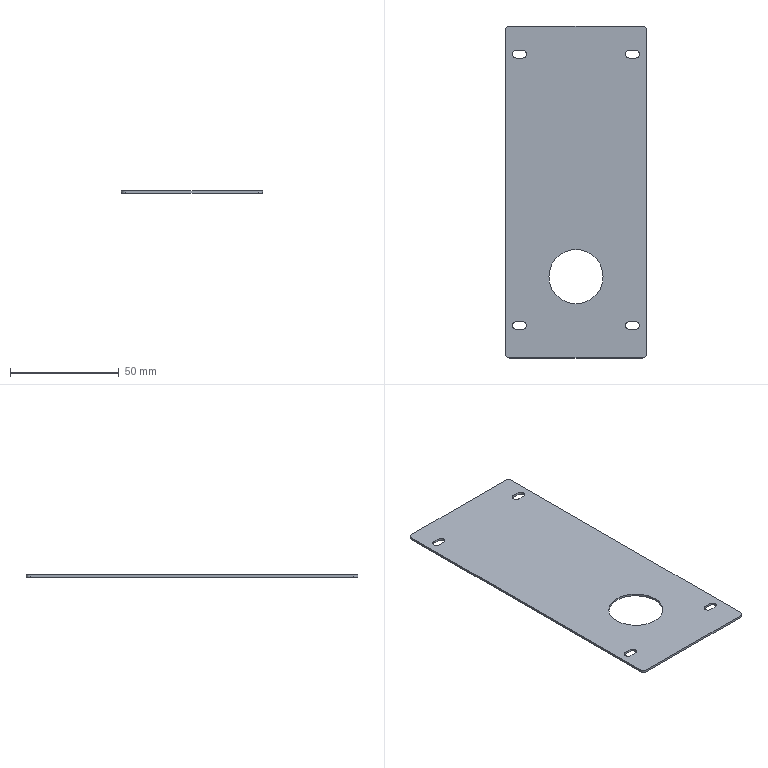Part | STEP file | cover plate 1 | 1 solid | 32 faces | box 65 x 153 x 1 mm | volume 9370 mm3 | cylinder 18 | plane 14 | commonest cylinder face diameters 3.5 x12 4 x4 25 x2